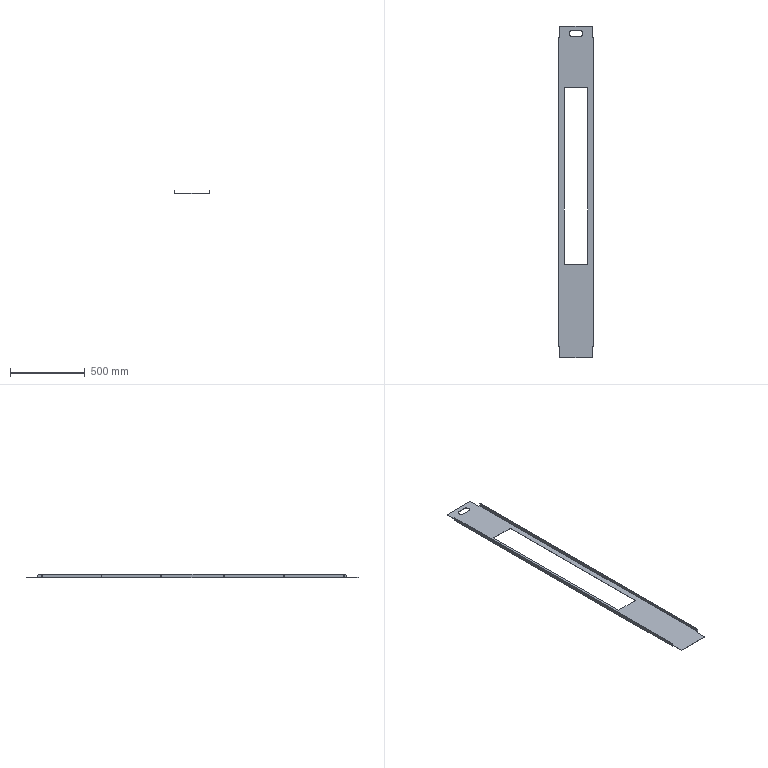Part | SolidWorks | features Chamfer 2, Cut 2, ICE 2, FlatPattern 1, SMBaseFlange 1, SheetMetal 1 | 1 solid | 69 faces | box 240 x 2216 x 23 mm | volume 637651 mm3 | plane 38 | cylinder 31 | commonest cylinder face diameters 6.2 x24 40 x3 0.4 x2 3.4 x2